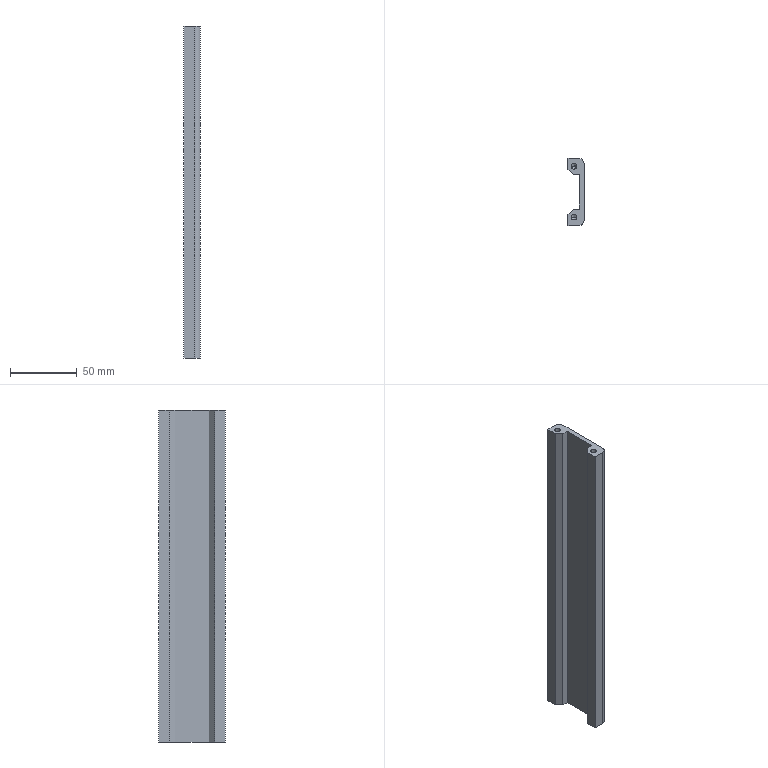Part | STEP file | 1 solid | 30 faces | box 12 x 50 x 248 mm | volume 87500 mm3 | plane 12 | cylinder 10 | cone 8 | commonest cylinder face diameters 4.2 x8 8 x2